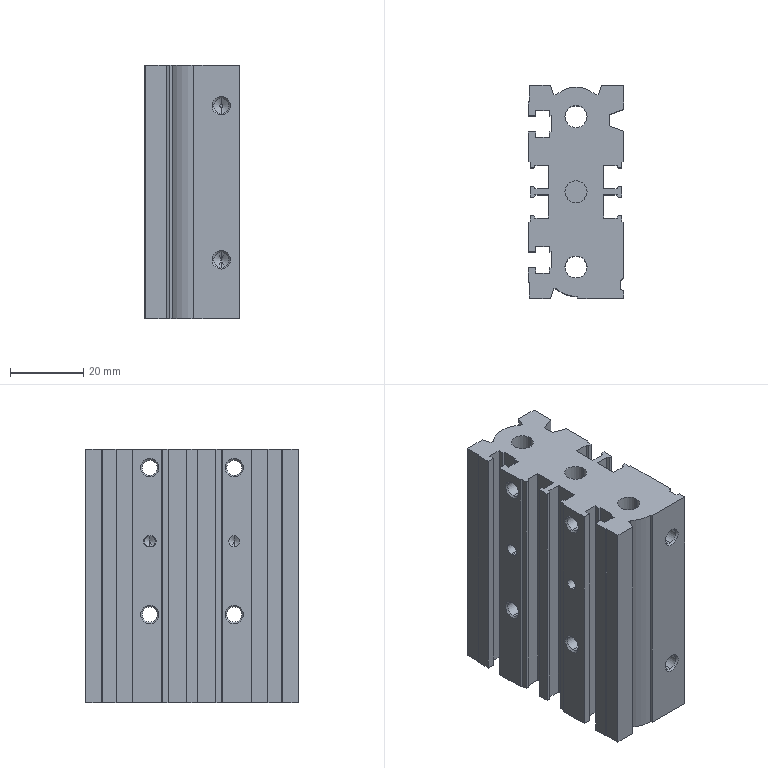Part | SolidWorks | features RevCut 16, RefAxis 15, ICE 10, 3DProfileFeature 5, Extrusion 1 | 1 solid | 219 faces | box 26 x 58 x 69 mm | volume 73363 mm3 | plane 117 | cylinder 62 | cone 40 | commonest cylinder face diameters 4.134 x16 3 x12 3.242 x8 4.3 x8 8 x8 6 x6